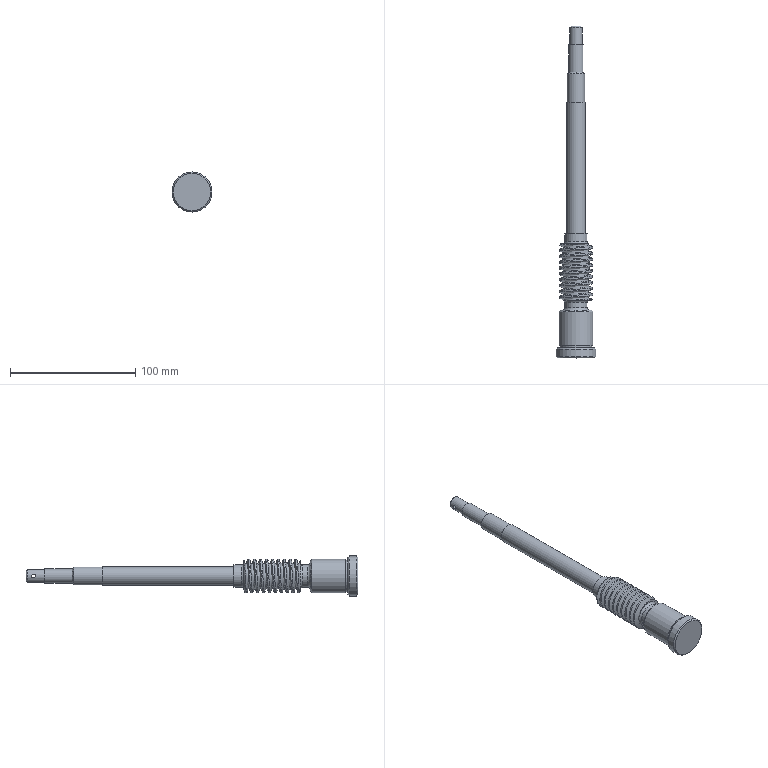Part | NX | features DATUM_CSYS 4, SKETCH 3, BLEND 1, CHAMFER 1, EXTRUDE 1, HELIX 1, OFFSET_REGION 1, SKIN 1, SUBTRACT 1, SWP104 1, SYMBOLIC_THREAD 1 | 1 solid | 35 faces | box 32 x 265 x 32 mm | volume 73898 mm3 | plane 12 | cylinder 11 | cone 7 | torus 3 | spline 2 | commonest cylinder face diameters 18 x2 3 x1 10 x1 11.5 x1 14 x1 15 x1